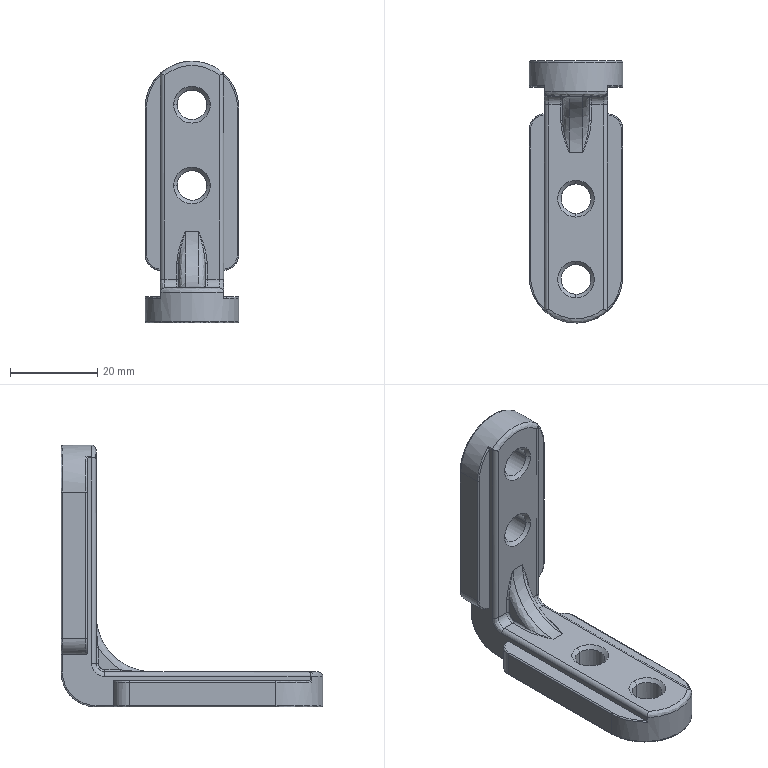Part | STEP file | 46A-01009CC13 | 1 solid | 95 faces | box 21.5 x 60 x 60 mm | volume 15069 mm3 | cylinder 42 | spline 29 | plane 16 | other 8 | commonest cylinder face diameters 0.6 x16 6.8 x8 1 x4 2 x4 7.5 x4 4 x2